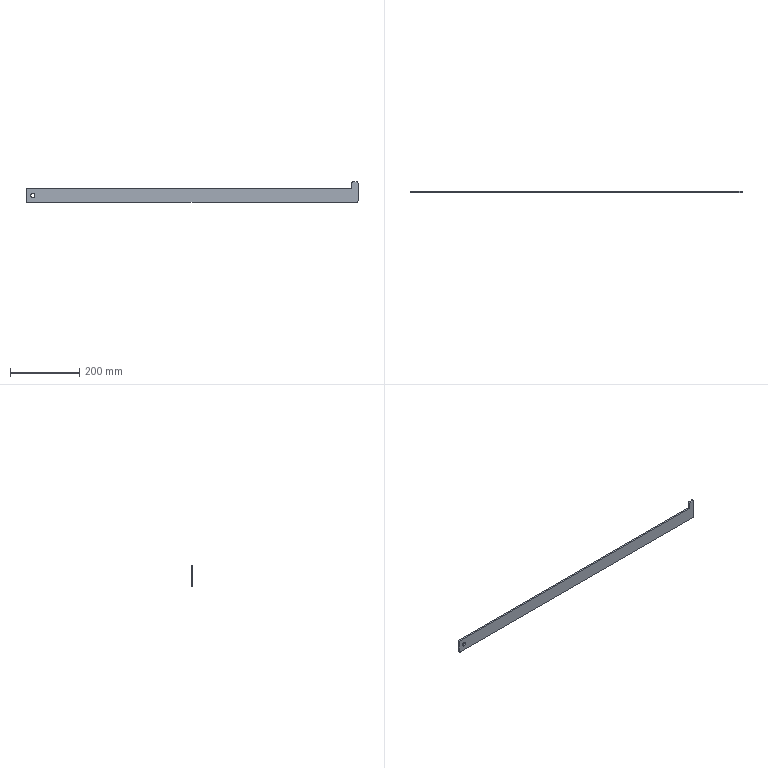Part | SolidWorks | features ICE 2, Fillet 1, FlatPattern 1, SMBaseFlange 1, SheetMetal 1 | 1 solid | 15 faces | box 960 x 5 x 60 mm | volume 193100 mm3 | plane 8 | cylinder 7 | commonest cylinder face diameters 10 x5 12 x2
STEP:
#1=CARTESIAN_POINT('',(-460.,-5.,6.));
#2=VERTEX_POINT('',#1);
#3=CARTESIAN_POINT('',(-460.,-5.,-6.));
#4=VERTEX_POINT('',#3);
#5=CARTESIAN_POINT('',(-460.,-5.,0.));
#6=DIRECTION('',(0.,-1.,0.));
#7=DIRECTION('',(0.,0.,-1.));
#8=AXIS2_PLACEMENT_3D('',#5,#6,#7);
#9=CIRCLE('',#8,6.);
#10=EDGE_CURVE('',#2,#4,#9,.T.);
#11=ORIENTED_EDGE('',*,*,#10,.T.);
#12=CARTESIAN_POINT('',(-460.,0.,-6.));
#13=VERTEX_POINT('',#12);
#14=CARTESIAN_POINT('',(-460.,-10.,-6.));
#15=DIRECTION('',(0.,1.,0.));
#16=VECTOR('',#15,1000.);
#17=LINE('',#14,#16);
#18=EDGE_CURVE('',#4,#13,#17,.T.);
#19=ORIENTED_EDGE('',*,*,#18,.T.);
#20=CARTESIAN_POINT('',(-460.,0.,6.));
#21=VERTEX_POINT('',#20);
#22=CARTESIAN_POINT('',(-460.,0.,0.));
#23=DIRECTION('',(0.,1.,0.));
#24=DIRECTION('',(0.,0.,1.));
#25=AXIS2_PLACEMENT_3D('',#22,#23,#24);
#26=CIRCLE('',#25,6.);
#27=EDGE_CURVE('',#13,#21,#26,.T.);
#28=ORIENTED_EDGE('',*,*,#27,.T.);
#29=CARTESIAN_POINT('',(-460.,-10.,6.));
#30=DIRECTION('',(0.,1.,0.));
#31=VECTOR('',#30,1000.);
#32=LINE('',#29,#31);
#33=EDGE_CURVE('',#2,#21,#32,.T.);
#34=ORIENTED_EDGE('',*,*,#33,.F.);
#35=EDGE_LOOP('',(#11,#19,#28,#34));
#36=FACE_OUTER_BOUND('',#35,.T.);
#37=CARTESIAN_POINT('',(-460.,-10.,0.));
#38=DIRECTION('',(0.,1.,0.));
#39=DIRECTION('',(0.,0.,1.));
#40=AXIS2_PLACEMENT_3D('',#37,#38,#39);
#41=CYLINDRICAL_SURFACE('',#40,6.);
#42=ADVANCED_FACE('',(#36),#41,.F.);
#43=CARTESIAN_POINT('',(-475.,0.,20.));
#44=VERTEX_POINT('',#43);
#45=CARTESIAN_POINT('',(462.,0.,20.));
#46=VERTEX_POINT('',#45);
#47=CARTESIAN_POINT('',(-480.,0.,20.));
#48=DIRECTION('',(1.,0.,0.));
#49=VECTOR('',#48,1000.);
#50=LINE('',#47,#49);
#51=EDGE_CURVE('',#44,#46,#50,.T.);
#52=ORIENTED_EDGE('',*,*,#51,.F.);
#53=CARTESIAN_POINT('',(-475.,-5.,20.));
#54=VERTEX_POINT('',#53);
#55=CARTESIAN_POINT('',(-475.,-5.,20.));
#56=DIRECTION('',(0.,-1.,0.));
#57=VECTOR('',#56,1000.);
#58=LINE('',#55,#57);
#59=EDGE_CURVE('',#44,#54,#58,.T.);
#60=ORIENTED_EDGE('',*,*,#59,.T.);
#61=CARTESIAN_POINT('',(462.,-5.,20.));
#62=VERTEX_POINT('',#61);
#63=CARTESIAN_POINT('',(-480.,-5.,20.));
#64=DIRECTION('',(1.,0.,0.));
#65=VECTOR('',#64,1000.);
#66=LINE('',#63,#65);
#67=EDGE_CURVE('',#54,#62,#66,.T.);
#68=ORIENTED_EDGE('',*,*,#67,.T.);
#69=CARTESIAN_POINT('',(462.,-5.,20.));
#70=DIRECTION('',(0.,1.,0.));
#71=VECTOR('',#70,1000.);
#72=LINE('',#69,#71);
#73=EDGE_CURVE('',#62,#46,#72,.T.);
#74=ORIENTED_EDGE('',*,*,#73,.T.);
#75=EDGE_LOOP('',(#52,#60,#68,#74));
#76=FACE_OUTER_BOUND('',#75,.T.);
#77=CARTESIAN_POINT('',(-480.,-5.,20.));
#78=DIRECTION('',(0.,0.,1.));
#79=DIRECTION('',(1.,0.,0.));
#80=AXIS2_PLACEMENT_3D('',#77,#78,#79);
#81=PLANE('',#80);
#82=ADVANCED_FACE('',(#76),#81,.T.);
#83=CARTESIAN_POINT('',(480.,-5.,35.));
#84=VERTEX_POINT('',#83);
#85=CARTESIAN_POINT('',(480.,-5.,-15.));
#86=VERTEX_POINT('',#85);
#87=CARTESIAN_POINT('',(480.,-5.,20.));
#88=DIRECTION('',(0.,0.,-1.));
#89=VECTOR('',#88,1000.);
#90=LINE('',#87,#89);
#91=EDGE_CURVE('',#84,#86,#90,.T.);
#92=ORIENTED_EDGE('',*,*,#91,.T.);
#93=CARTESIAN_POINT('',(480.,0.,-15.));
#94=VERTEX_POINT('',#93);
#95=CARTESIAN_POINT('',(480.,-5.,-15.));
#96=DIRECTION('',(0.,1.,0.));
#97=VECTOR('',#96,1000.);
#98=LINE('',#95,#97);
#99=EDGE_CURVE('',#86,#94,#98,.T.);
#100=ORIENTED_EDGE('',*,*,#99,.T.);
#101=CARTESIAN_POINT('',(480.,0.,35.));
#102=VERTEX_POINT('',#101);
#103=CARTESIAN_POINT('',(480.,0.,20.));
#104=DIRECTION('',(0.,0.,-1.));
#105=VECTOR('',#104,1000.);
#106=LINE('',#103,#105);
#107=EDGE_CURVE('',#102,#94,#106,.T.);
#108=ORIENTED_EDGE('',*,*,#107,.F.);
#109=CARTESIAN_POINT('',(480.,-5.,35.));
#110=DIRECTION('',(0.,-1.,0.));
#111=VECTOR('',#110,1000.);
#112=LINE('',#109,#111);
#113=EDGE_CURVE('',#102,#84,#112,.T.);
#114=ORIENTED_EDGE('',*,*,#113,.T.);
#115=EDGE_LOOP('',(#92,#100,#108,#114));
#116=FACE_OUTER_BOUND('',#115,.T.);
#117=CARTESIAN_POINT('',(480.,-5.,20.));
#118=DIRECTION('',(1.,0.,0.));
#119=DIRECTION('',(0.,0.,-1.));
#120=AXIS2_PLACEMENT_3D('',#117,#118,#119);
#121=PLANE('',#120);
#122=ADVANCED_FACE('',(#116),#121,.T.);
#123=CARTESIAN_POINT('',(-480.,0.,-15.));
#124=VERTEX_POINT('',#123);
#125=CARTESIAN_POINT('',(-480.,0.,15.));
#126=VERTEX_POINT('',#125);
#127=CARTESIAN_POINT('',(-480.,0.,20.));
#128=DIRECTION('',(0.,0.,1.));
#129=VECTOR('',#128,1000.);
#130=LINE('',#127,#129);
#131=EDGE_CURVE('',#124,#126,#130,.T.);
#132=ORIENTED_EDGE('',*,*,#131,.F.);
#133=CARTESIAN_POINT('',(-480.,-5.,-15.));
#134=VERTEX_POINT('',#133);
#135=CARTESIAN_POINT('',(-480.,-5.,-15.));
#136=DIRECTION('',(0.,-1.,0.));
#137=VECTOR('',#136,1000.);
#138=LINE('',#135,#137);
#139=EDGE_CURVE('',#124,#134,#138,.T.);
#140=ORIENTED_EDGE('',*,*,#139,.T.);
#141=CARTESIAN_POINT('',(-480.,-5.,15.));
#142=VERTEX_POINT('',#141);
#143=CARTESIAN_POINT('',(-480.,-5.,20.));
#144=DIRECTION('',(0.,0.,1.));
#145=VECTOR('',#144,1000.);
#146=LINE('',#143,#145);
#147=EDGE_CURVE('',#134,#142,#146,.T.);
#148=ORIENTED_EDGE('',*,*,#147,.T.);
#149=CARTESIAN_POINT('',(-480.,-5.,15.));
#150=DIRECTION('',(0.,1.,0.));
#151=VECTOR('',#150,1000.);
#152=LINE('',#149,#151);
#153=EDGE_CURVE('',#142,#126,#152,.T.);
#154=ORIENTED_EDGE('',*,*,#153,.T.);
#155=EDGE_LOOP('',(#132,#140,#148,#154));
#156=FACE_OUTER_BOUND('',#155,.T.);
#157=CARTESIAN_POINT('',(-480.,-5.,20.));
#158=DIRECTION('',(-1.,0.,0.));
#159=DIRECTION('',(0.,0.,1.));
#160=AXIS2_PLACEMENT_3D('',#157,#158,#159);
#161=PLANE('',#160);
#162=ADVANCED_FACE('',(#156),#161,.T.);
#163=CARTESIAN_POINT('',(475.,0.,-20.));
#164=VERTEX_POINT('',#163);
#165=CARTESIAN_POINT('',(-475.,0.,-20.));
#166=VERTEX_POINT('',#165);
#167=CARTESIAN_POINT('',(-480.,0.,-20.));
#168=DIRECTION('',(-1.,0.,0.));
#169=VECTOR('',#168,1000.);
#170=LINE('',#167,#169);
#171=EDGE_CURVE('',#164,#166,#170,.T.);
#172=ORIENTED_EDGE('',*,*,#171,.F.);
#173=CARTESIAN_POINT('',(475.,-5.,-20.));
#174=VERTEX_POINT('',#173);
#175=CARTESIAN_POINT('',(475.,-5.,-20.));
#176=DIRECTION('',(0.,-1.,0.));
#177=VECTOR('',#176,1000.);
#178=LINE('',#175,#177);
#179=EDGE_CURVE('',#164,#174,#178,.T.);
#180=ORIENTED_EDGE('',*,*,#179,.T.);
#181=CARTESIAN_POINT('',(-475.,-5.,-20.));
#182=VERTEX_POINT('',#181);
#183=CARTESIAN_POINT('',(-480.,-5.,-20.));
#184=DIRECTION('',(-1.,0.,0.));
#185=VECTOR('',#184,1000.);
#186=LINE('',#183,#185);
#187=EDGE_CURVE('',#174,#182,#186,.T.);
#188=ORIENTED_EDGE('',*,*,#187,.T.);
#189=CARTESIAN_POINT('',(-475.,-5.,-20.));
#190=DIRECTION('',(0.,1.,0.));
#191=VECTOR('',#190,1000.);
#192=LINE('',#189,#191);
#193=EDGE_CURVE('',#182,#166,#192,.T.);
#194=ORIENTED_EDGE('',*,*,#193,.T.);
#195=EDGE_LOOP('',(#172,#180,#188,#194));
#196=FACE_OUTER_BOUND('',#195,.T.);
#197=CARTESIAN_POINT('',(-480.,-5.,-20.));
#198=DIRECTION('',(0.,0.,-1.));
#199=DIRECTION('',(-1.,0.,0.));
#200=AXIS2_PLACEMENT_3D('',#197,#198,#199);
#201=PLANE('',#200);
#202=ADVANCED_FACE('',(#196),#201,.T.);
#203=ORIENTED_EDGE('',*,*,#10,.F.);
#204=CARTESIAN_POINT('',(-460.,-5.,0.));
#205=DIRECTION('',(0.,-1.,0.));
#206=DIRECTION('',(0.,0.,-1.));
#207=AXIS2_PLACEMENT_3D('',#204,#205,#206);
#208=CIRCLE('',#207,6.);
#209=EDGE_CURVE('',#4,#2,#208,.T.);
#210=ORIENTED_EDGE('',*,*,#209,.F.);
#211=EDGE_LOOP('',(#203,#210));
#212=FACE_BOUND('',#211,.T.);
#213=ORIENTED_EDGE('',*,*,#187,.F.);
#214=CARTESIAN_POINT('',(475.,-5.,-15.));
#215=DIRECTION('',(0.,-1.,0.));
#216=DIRECTION('',(0.,0.,-1.));
#217=AXIS2_PLACEMENT_3D('',#214,#215,#216);
#218=CIRCLE('',#217,5.);
#219=EDGE_CURVE('',#174,#86,#218,.T.);
#220=ORIENTED_EDGE('',*,*,#219,.T.);
#221=ORIENTED_EDGE('',*,*,#91,.F.);
#222=CARTESIAN_POINT('',(475.,-5.,40.));
#223=VERTEX_POINT('',#222);
#224=CARTESIAN_POINT('',(475.,-5.,35.));
#225=DIRECTION('',(0.,-1.,0.));
#226=DIRECTION('',(0.,0.,-1.));
#227=AXIS2_PLACEMENT_3D('',#224,#225,#226);
#228=CIRCLE('',#227,5.);
#229=EDGE_CURVE('',#84,#223,#228,.T.);
#230=ORIENTED_EDGE('',*,*,#229,.T.);
#231=CARTESIAN_POINT('',(467.,-5.,40.));
#232=VERTEX_POINT('',#231);
#233=CARTESIAN_POINT('',(480.,-5.,40.));
#234=DIRECTION('',(1.,0.,0.));
#235=VECTOR('',#234,1000.);
#236=LINE('',#233,#235);
#237=EDGE_CURVE('',#232,#223,#236,.T.);
#238=ORIENTED_EDGE('',*,*,#237,.F.);
#239=CARTESIAN_POINT('',(462.,-5.,35.));
#240=VERTEX_POINT('',#239);
#241=CARTESIAN_POINT('',(467.,-5.,35.));
#242=DIRECTION('',(0.,-1.,0.));
#243=DIRECTION('',(0.,0.,-1.));
#244=AXIS2_PLACEMENT_3D('',#241,#242,#243);
#245=CIRCLE('',#244,5.);
#246=EDGE_CURVE('',#232,#240,#245,.T.);
#247=ORIENTED_EDGE('',*,*,#246,.T.);
#248=CARTESIAN_POINT('',(462.,-5.,20.));
#249=DIRECTION('',(0.,0.,1.));
#250=VECTOR('',#249,1000.);
#251=LINE('',#248,#250);
#252=EDGE_CURVE('',#62,#240,#251,.T.);
#253=ORIENTED_EDGE('',*,*,#252,.F.);
#254=ORIENTED_EDGE('',*,*,#67,.F.);
#255=CARTESIAN_POINT('',(-475.,-5.,15.));
#256=DIRECTION('',(0.,-1.,0.));
#257=DIRECTION('',(0.,0.,-1.));
#258=AXIS2_PLACEMENT_3D('',#255,#256,#257);
#259=CIRCLE('',#258,5.);
#260=EDGE_CURVE('',#54,#142,#259,.T.);
#261=ORIENTED_EDGE('',*,*,#260,.T.);
#262=ORIENTED_EDGE('',*,*,#147,.F.);
#263=CARTESIAN_POINT('',(-475.,-5.,-15.));
#264=DIRECTION('',(0.,-1.,0.));
#265=DIRECTION('',(0.,0.,-1.));
#266=AXIS2_PLACEMENT_3D('',#263,#264,#265);
#267=CIRCLE('',#266,5.);
#268=EDGE_CURVE('',#134,#182,#267,.T.);
#269=ORIENTED_EDGE('',*,*,#268,.T.);
#270=EDGE_LOOP('',(#213,#220,#221,#230,#238,#247,#253,#254,#261,#262,#269));
#271=FACE_OUTER_BOUND('',#270,.T.);
#272=CARTESIAN_POINT('',(0.,-5.,0.));
#273=DIRECTION('',(0.,-1.,0.));
#274=DIRECTION('',(0.,0.,-1.));
#275=AXIS2_PLACEMENT_3D('',#272,#273,#274);
#276=PLANE('',#275);
#277=ADVANCED_FACE('',(#212,#271),#276,.T.);
#278=CARTESIAN_POINT('',(-460.,0.,0.));
#279=DIRECTION('',(0.,1.,0.));
#280=DIRECTION('',(0.,0.,1.));
#281=AXIS2_PLACEMENT_3D('',#278,#279,#280);
#282=CIRCLE('',#281,6.);
#283=EDGE_CURVE('',#21,#13,#282,.T.);
#284=ORIENTED_EDGE('',*,*,#283,.F.);
#285=ORIENTED_EDGE('',*,*,#27,.F.);
#286=EDGE_LOOP('',(#284,#285));
#287=FACE_BOUND('',#286,.T.);
#288=ORIENTED_EDGE('',*,*,#107,.T.);
#289=CARTESIAN_POINT('',(475.,0.,-15.));
#290=DIRECTION('',(0.,1.,0.));
#291=DIRECTION('',(0.,0.,-1.));
#292=AXIS2_PLACEMENT_3D('',#289,#290,#291);
#293=CIRCLE('',#292,5.);
#294=EDGE_CURVE('',#94,#164,#293,.T.);
#295=ORIENTED_EDGE('',*,*,#294,.T.);
#296=ORIENTED_EDGE('',*,*,#171,.T.);
#297=CARTESIAN_POINT('',(-475.,0.,-15.));
#298=DIRECTION('',(0.,1.,0.));
#299=DIRECTION('',(0.,0.,-1.));
#300=AXIS2_PLACEMENT_3D('',#297,#298,#299);
#301=CIRCLE('',#300,5.);
#302=EDGE_CURVE('',#166,#124,#301,.T.);
#303=ORIENTED_EDGE('',*,*,#302,.T.);
#304=ORIENTED_EDGE('',*,*,#131,.T.);
#305=CARTESIAN_POINT('',(-475.,0.,15.));
#306=DIRECTION('',(0.,1.,0.));
#307=DIRECTION('',(0.,0.,-1.));
#308=AXIS2_PLACEMENT_3D('',#305,#306,#307);
#309=CIRCLE('',#308,5.);
#310=EDGE_CURVE('',#126,#44,#309,.T.);
#311=ORIENTED_EDGE('',*,*,#310,.T.);
#312=ORIENTED_EDGE('',*,*,#51,.T.);
#313=CARTESIAN_POINT('',(462.,0.,35.));
#314=VERTEX_POINT('',#313);
#315=CARTESIAN_POINT('',(462.,0.,20.));
#316=DIRECTION('',(0.,0.,1.));
#317=VECTOR('',#316,1000.);
#318=LINE('',#315,#317);
#319=EDGE_CURVE('',#46,#314,#318,.T.);
#320=ORIENTED_EDGE('',*,*,#319,.T.);
#321=CARTESIAN_POINT('',(467.,0.,40.));
#322=VERTEX_POINT('',#321);
#323=CARTESIAN_POINT('',(467.,0.,35.));
#324=DIRECTION('',(0.,1.,0.));
#325=DIRECTION('',(0.,0.,-1.));
#326=AXIS2_PLACEMENT_3D('',#323,#324,#325);
#327=CIRCLE('',#326,5.);
#328=EDGE_CURVE('',#314,#322,#327,.T.);
#329=ORIENTED_EDGE('',*,*,#328,.T.);
#330=CARTESIAN_POINT('',(475.,0.,40.));
#331=VERTEX_POINT('',#330);
#332=CARTESIAN_POINT('',(480.,0.,40.));
#333=DIRECTION('',(1.,0.,0.));
#334=VECTOR('',#333,1000.);
#335=LINE('',#332,#334);
#336=EDGE_CURVE('',#322,#331,#335,.T.);
#337=ORIENTED_EDGE('',*,*,#336,.T.);
#338=CARTESIAN_POINT('',(475.,0.,35.));
#339=DIRECTION('',(0.,1.,0.));
#340=DIRECTION('',(0.,0.,-1.));
#341=AXIS2_PLACEMENT_3D('',#338,#339,#340);
#342=CIRCLE('',#341,5.);
#343=EDGE_CURVE('',#331,#102,#342,.T.);
#344=ORIENTED_EDGE('',*,*,#343,.T.);
#345=EDGE_LOOP('',(#288,#295,#296,#303,#304,#311,#312,#320,#329,#337,#344));
#346=FACE_OUTER_BOUND('',#345,.T.);
#347=CARTESIAN_POINT('',(0.,0.,0.));
#348=DIRECTION('',(0.,-1.,0.));
#349=DIRECTION('',(0.,0.,-1.));
#350=AXIS2_PLACEMENT_3D('',#347,#348,#349);
#351=PLANE('',#350);
#352=ADVANCED_FACE('',(#287,#346),#351,.F.);
#353=ORIENTED_EDGE('',*,*,#18,.F.);
#354=ORIENTED_EDGE('',*,*,#209,.T.);
#355=ORIENTED_EDGE('',*,*,#33,.T.);
#356=ORIENTED_EDGE('',*,*,#283,.T.);
#357=EDGE_LOOP('',(#353,#354,#355,#356));
#358=FACE_OUTER_BOUND('',#357,.T.);
#359=CARTESIAN_POINT('',(-460.,-10.,0.));
#360=DIRECTION('',(0.,1.,0.));
#361=DIRECTION('',(0.,0.,1.));
#362=AXIS2_PLACEMENT_3D('',#359,#360,#361);
#363=CYLINDRICAL_SURFACE('',#362,6.);
#364=ADVANCED_FACE('',(#358),#363,.F.);
#365=ORIENTED_EDGE('',*,*,#237,.T.);
#366=CARTESIAN_POINT('',(475.,-5.,40.));
#367=DIRECTION('',(0.,1.,0.));
#368=VECTOR('',#367,1000.);
#369=LINE('',#366,#368);
#370=EDGE_CURVE('',#223,#331,#369,.T.);
#371=ORIENTED_EDGE('',*,*,#370,.T.);
#372=ORIENTED_EDGE('',*,*,#336,.F.);
#373=CARTESIAN_POINT('',(467.,-5.,40.));
#374=DIRECTION('',(0.,-1.,0.));
#375=VECTOR('',#374,1000.);
#376=LINE('',#373,#375);
#377=EDGE_CURVE('',#322,#232,#376,.T.);
#378=ORIENTED_EDGE('',*,*,#377,.T.);
#379=EDGE_LOOP('',(#365,#371,#372,#378));
#380=FACE_OUTER_BOUND('',#379,.T.);
#381=CARTESIAN_POINT('',(480.,-5.,40.));
#382=DIRECTION('',(0.,0.,1.));
#383=DIRECTION('',(1.,0.,0.));
#384=AXIS2_PLACEMENT_3D('',#381,#382,#383);
#385=PLANE('',#384);
#386=ADVANCED_FACE('',(#380),#385,.T.);
#387=ORIENTED_EDGE('',*,*,#252,.T.);
#388=CARTESIAN_POINT('',(462.,-5.,35.));
#389=DIRECTION('',(0.,1.,0.));
#390=VECTOR('',#389,1000.);
#391=LINE('',#388,#390);
#392=EDGE_CURVE('',#240,#314,#391,.T.);
#393=ORIENTED_EDGE('',*,*,#392,.T.);
#394=ORIENTED_EDGE('',*,*,#319,.F.);
#395=ORIENTED_EDGE('',*,*,#73,.F.);
#396=EDGE_LOOP('',(#387,#393,#394,#395));
#397=FACE_OUTER_BOUND('',#396,.T.);
#398=CARTESIAN_POINT('',(462.,-5.,20.));
#399=DIRECTION('',(-1.,0.,0.));
#400=DIRECTION('',(0.,0.,1.));
#401=AXIS2_PLACEMENT_3D('',#398,#399,#400);
#402=PLANE('',#401);
#403=ADVANCED_FACE('',(#397),#402,.T.);
#404=ORIENTED_EDGE('',*,*,#219,.F.);
#405=ORIENTED_EDGE('',*,*,#179,.F.);
#406=ORIENTED_EDGE('',*,*,#294,.F.);
#407=ORIENTED_EDGE('',*,*,#99,.F.);
#408=EDGE_LOOP('',(#404,#405,#406,#407));
#409=FACE_OUTER_BOUND('',#408,.T.);
#410=CARTESIAN_POINT('',(475.,-5.,-15.));
#411=DIRECTION('',(0.,1.,0.));
#412=DIRECTION('',(0.,0.,1.));
#413=AXIS2_PLACEMENT_3D('',#410,#411,#412);
#414=CYLINDRICAL_SURFACE('',#413,5.);
#415=ADVANCED_FACE('',(#409),#414,.T.);
#416=ORIENTED_EDGE('',*,*,#268,.F.);
#417=ORIENTED_EDGE('',*,*,#139,.F.);
#418=ORIENTED_EDGE('',*,*,#302,.F.);
#419=ORIENTED_EDGE('',*,*,#193,.F.);
#420=EDGE_LOOP('',(#416,#417,#418,#419));
#421=FACE_OUTER_BOUND('',#420,.T.);
#422=CARTESIAN_POINT('',(-475.,-5.,-15.));
#423=DIRECTION('',(0.,1.,0.));
#424=DIRECTION('',(0.,0.,1.));
#425=AXIS2_PLACEMENT_3D('',#422,#423,#424);
#426=CYLINDRICAL_SURFACE('',#425,5.);
#427=ADVANCED_FACE('',(#421),#426,.T.);
#428=ORIENTED_EDGE('',*,*,#260,.F.);
#429=ORIENTED_EDGE('',*,*,#59,.F.);
#430=ORIENTED_EDGE('',*,*,#310,.F.);
#431=ORIENTED_EDGE('',*,*,#153,.F.);
#432=EDGE_LOOP('',(#428,#429,#430,#431));
#433=FACE_OUTER_BOUND('',#432,.T.);
#434=CARTESIAN_POINT('',(-475.,-5.,15.));
#435=DIRECTION('',(0.,1.,0.));
#436=DIRECTION('',(0.,0.,1.));
#437=AXIS2_PLACEMENT_3D('',#434,#435,#436);
#438=CYLINDRICAL_SURFACE('',#437,5.);
#439=ADVANCED_FACE('',(#433),#438,.T.);
#440=ORIENTED_EDGE('',*,*,#229,.F.);
#441=ORIENTED_EDGE('',*,*,#113,.F.);
#442=ORIENTED_EDGE('',*,*,#343,.F.);
#443=ORIENTED_EDGE('',*,*,#370,.F.);
#444=EDGE_LOOP('',(#440,#441,#442,#443));
#445=FACE_OUTER_BOUND('',#444,.T.);
#446=CARTESIAN_POINT('',(475.,-5.,35.));
#447=DIRECTION('',(0.,1.,0.));
#448=DIRECTION('',(0.,0.,1.));
#449=AXIS2_PLACEMENT_3D('',#446,#447,#448);
#450=CYLINDRICAL_SURFACE('',#449,5.);
#451=ADVANCED_FACE('',(#445),#450,.T.);
#452=ORIENTED_EDGE('',*,*,#246,.F.);
#453=ORIENTED_EDGE('',*,*,#377,.F.);
#454=ORIENTED_EDGE('',*,*,#328,.F.);
#455=ORIENTED_EDGE('',*,*,#392,.F.);
#456=EDGE_LOOP('',(#452,#453,#454,#455));
#457=FACE_OUTER_BOUND('',#456,.T.);
#458=CARTESIAN_POINT('',(467.,-5.,35.));
#459=DIRECTION('',(0.,1.,0.));
#460=DIRECTION('',(0.,0.,1.));
#461=AXIS2_PLACEMENT_3D('',#458,#459,#460);
#462=CYLINDRICAL_SURFACE('',#461,5.);
#463=ADVANCED_FACE('',(#457),#462,.T.);
#464=CLOSED_SHELL('',(#42,#82,#122,#162,#202,#277,#352,#364,#386,#403,#415,#427,#439,#451,#463));
#465=MANIFOLD_SOLID_BREP('',#464);
#466=CARTESIAN_POINT('',(0.,0.,0.));
#467=DIRECTION('',(0.,0.,1.));
#468=DIRECTION('',(1.,0.,0.));
#469=AXIS2_PLACEMENT_3D('',#466,#467,#468);
#470=(LENGTH_UNIT()NAMED_UNIT(*)SI_UNIT(.MILLI.,.METRE.));
#471=UNCERTAINTY_MEASURE_WITH_UNIT(LENGTH_MEASURE(0.00001),#470,'','');
#472=(NAMED_UNIT(*)PLANE_ANGLE_UNIT()SI_UNIT($,.RADIAN.));
#473=(NAMED_UNIT(*)SI_UNIT($,.STERADIAN.)SOLID_ANGLE_UNIT());
#474=(GEOMETRIC_REPRESENTATION_CONTEXT(3)GLOBAL_UNCERTAINTY_ASSIGNED_CONTEXT((#471))GLOBAL_UNIT_ASSIGNED_CONTEXT((#470,#472,#473))REPRESENTATION_CONTEXT('',''));
#475=ADVANCED_BREP_SHAPE_REPRESENTATION('',(#465,#469),#474);